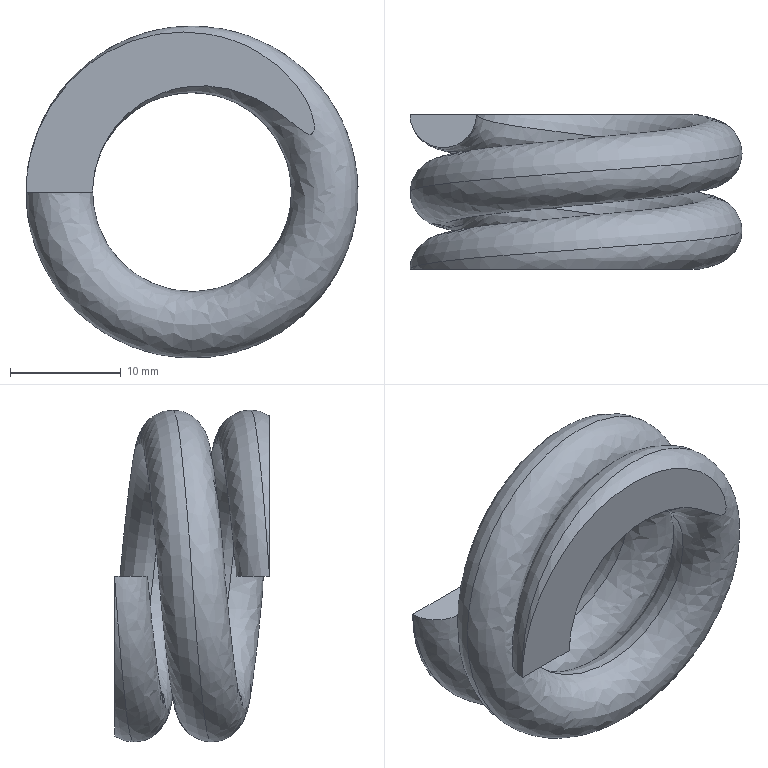Part | STEP file | Ejector spring 14 | 1 solid | 6 faces | box 30 x 14 x 30 mm | volume 3867 mm3 | plane 4 | spline 2